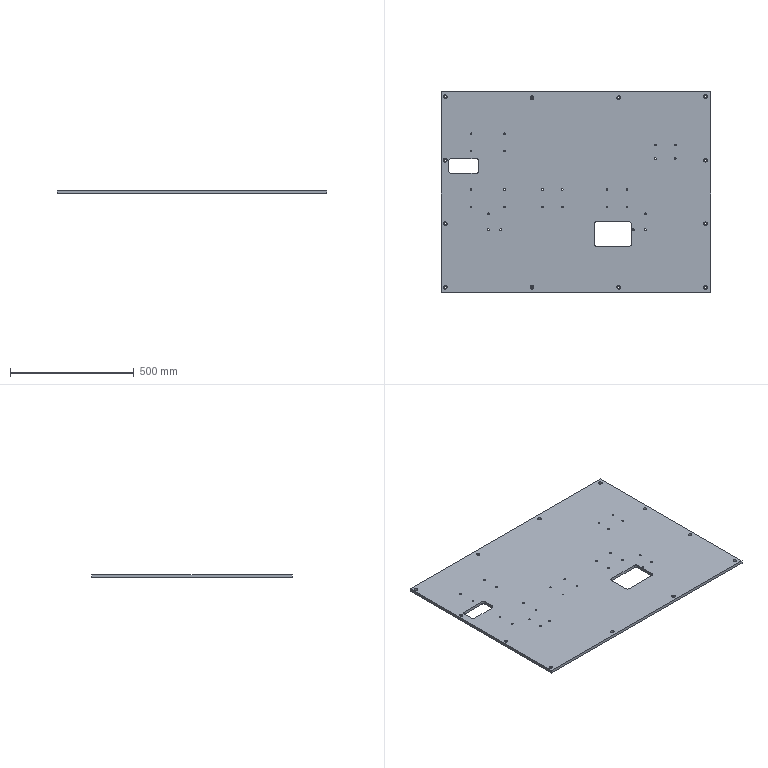Part | STEP file | X77-03001 | 1 solid | 134 faces | box 1087 x 810 x 12 mm | volume 10265289 mm3 | cylinder 108 | plane 26 | commonest cylinder face diameters 6.8 x52 9 x24 15 x24 20 x8